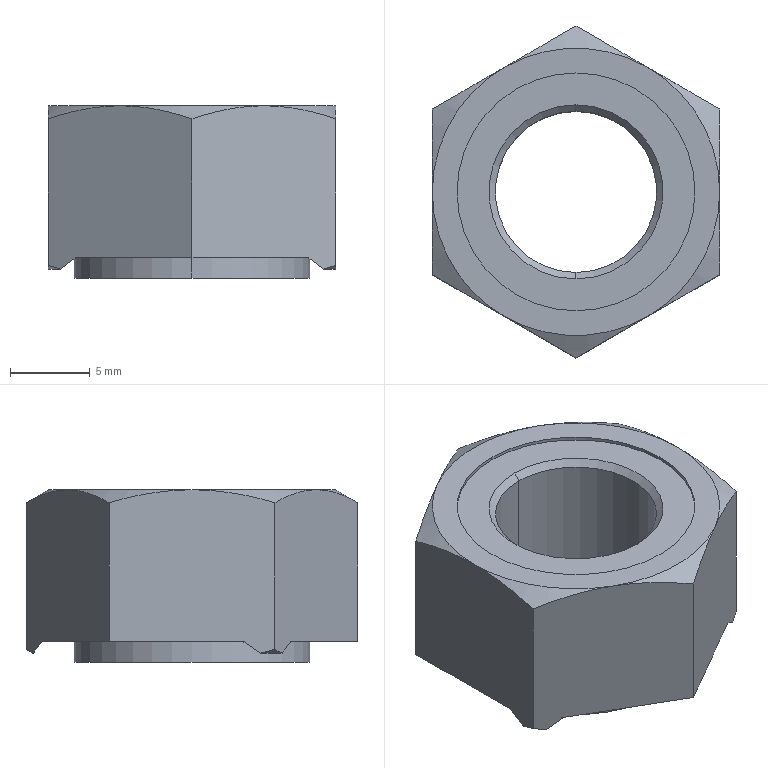Part | STEP file | 1 solid | 32 faces | box 18 x 20.785 x 10.8 mm | volume 1989 mm3 | cone 16 | plane 10 | cylinder 6 | commonest cylinder face diameters 10.106 x2 14.75 x2 14.9 x2